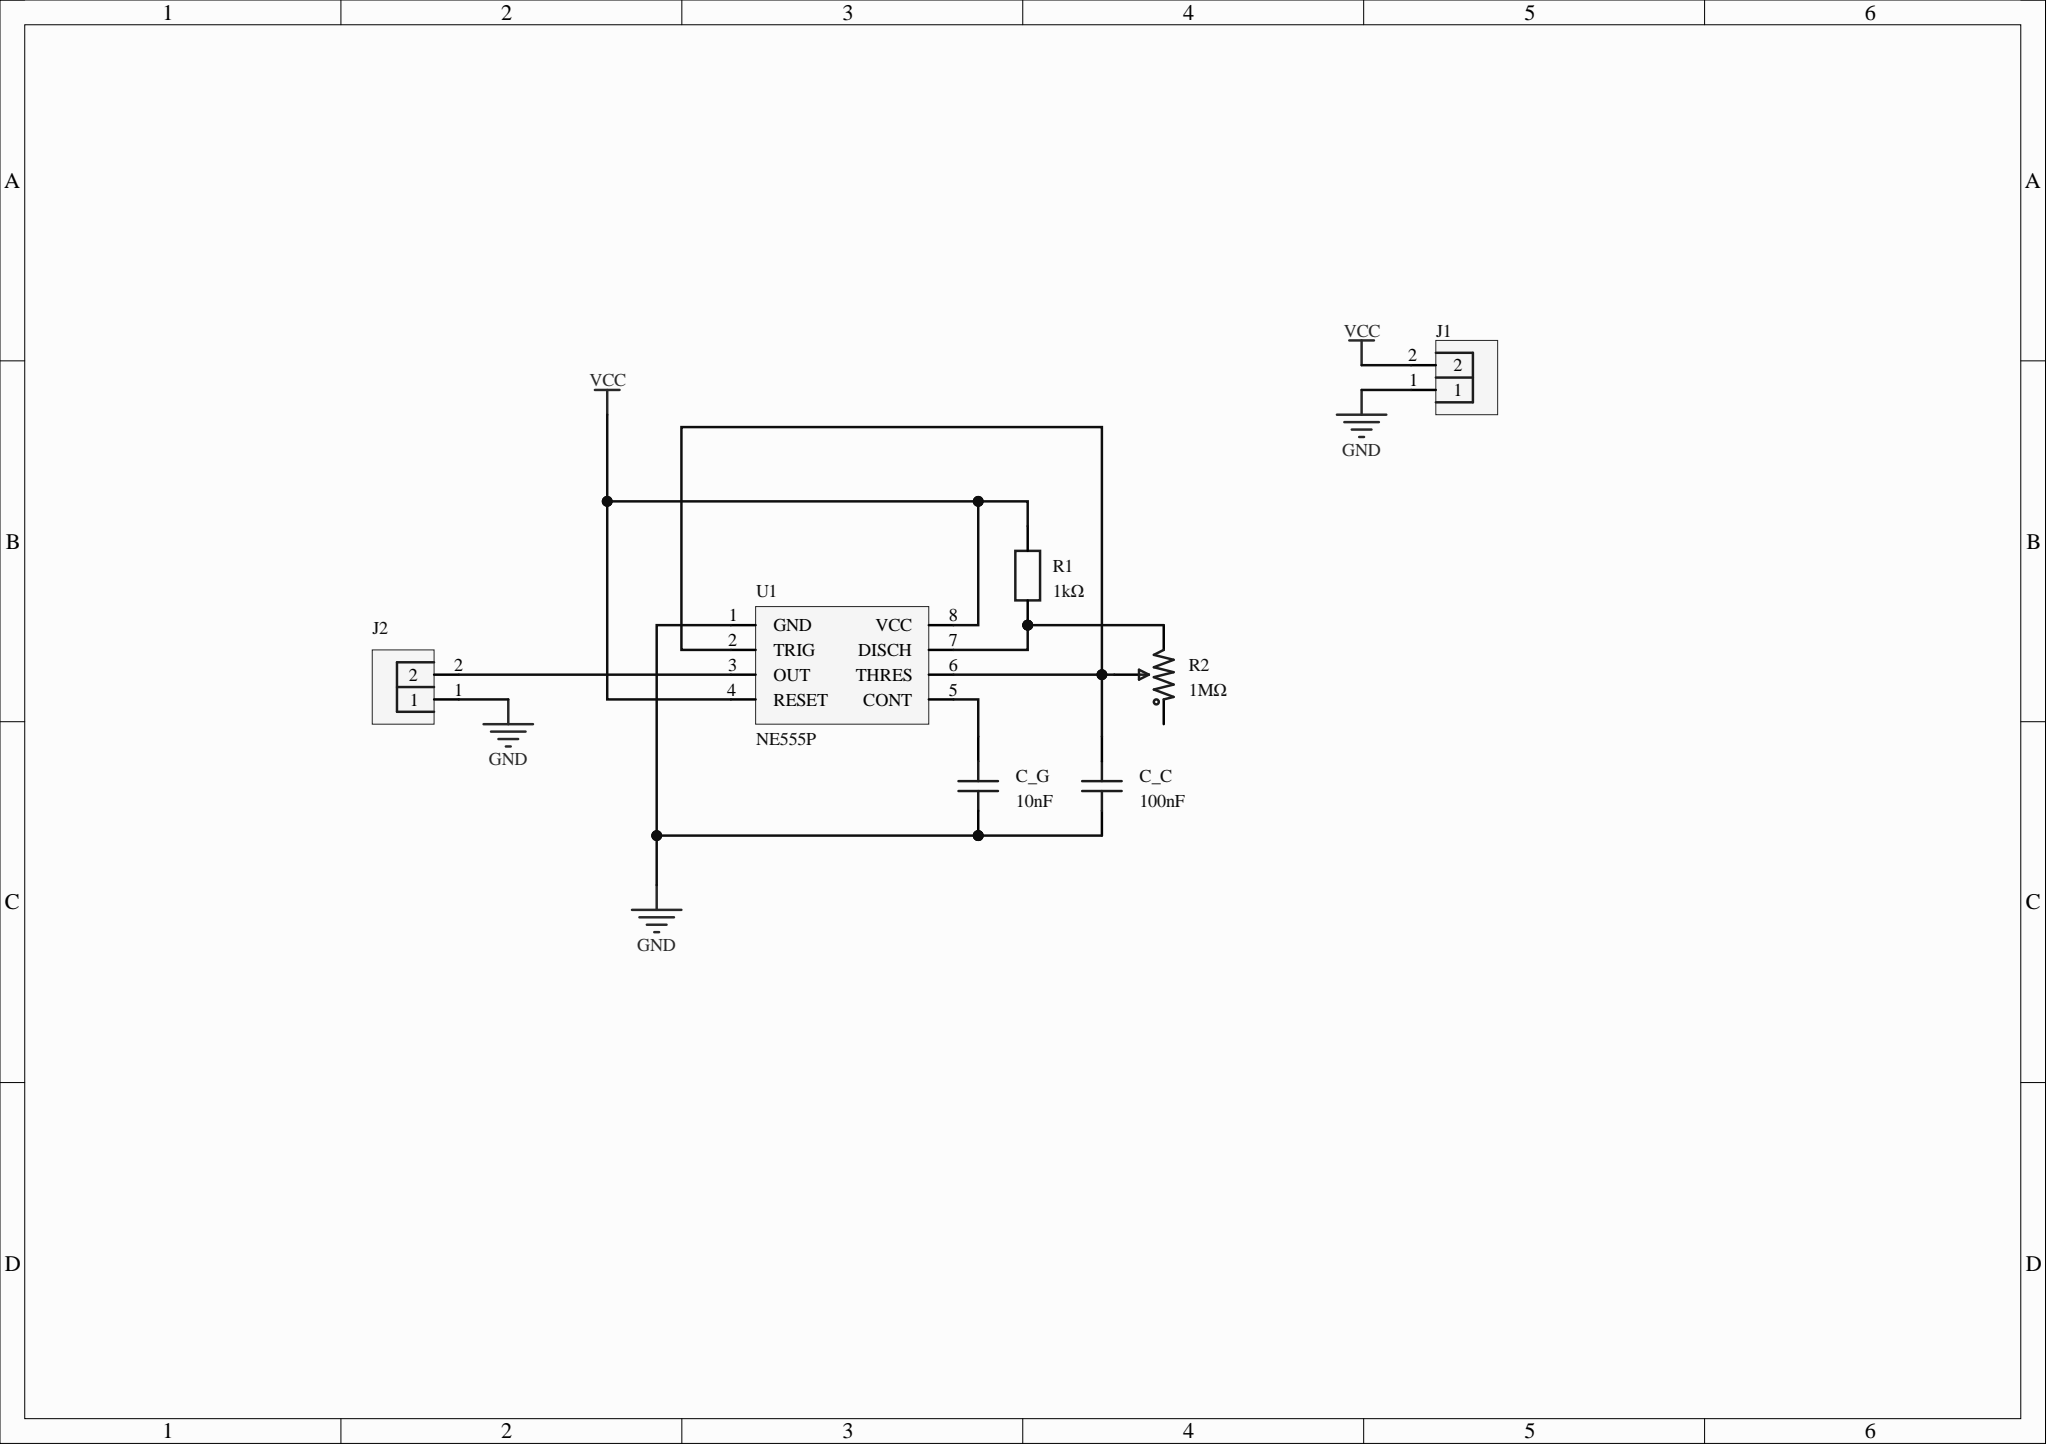Circuit board | Altium Designer | 7 parts | 6 nets
Bill of materials:
Comment,Description,Designator,Footprint,LibRef,Quantity
"100nF","Capacitance: 100nF; tolerance: ±20%; rated voltage: 50V; temperature coefficient: Y5V;","C_C","CAP-TH_L5.0-W2.5-P5.00-D1.0","CC1H104MC1FD3F6C10MF","1"
"10nF","Capacitance: 10nF; tolerance: ±20%; rated voltage: 50V; temperature coefficient: Y5U;","C_G","CAP-TH_L5.5-W3.0-P5.00-D0.6","DCT103M22Y5UF6FJ5A0","1"
"","","J1, J2","HDR-TH_2P-P2.54-V-M-1","HDR-M_2.54_1x2P","2"
"1kΩ","Resistor type: metal film resistor; resistance: 1kΩ; tolerance: ±1%; power: 250mW; temperature coefficient: ±100ppm/?;","R1","RES-TH_BD2.7-L6.2-P10.20-D0.4","MF1/4W-1K±1%-ST52","1"
"1MΩ","Resistance: 1MΩ; tolerance: ±25%; power: 100mW;","R2","RES-ADJ-TH_RM063-103","RM063-105(1M)","1"
"NE555P","Precision timing circuits that generate accurate time delays or oscillations. In delay or monostable mode, the timing interval is set by a single external resistor and capacitor network. In astable mode, frequency and duty cycle are set by two external resistors and one external capacitor.","U1","DIP-8_L9.8-W6.6-P2.54-LS7.6-BL","NE555P","1"
Netlist (Protel format):
[
C_C
CAP-TH_L5.0-W2.5-P5.00-D1.0
100nF



]
[
C_G
CAP-TH_L5.5-W3.0-P5.00-D0.6
10nF



]
[
J1
HDR-TH_2P-P2.54-V-M-1




]
[
J2
HDR-TH_2P-P2.54-V-M-1




]
[
R1
RES-TH_BD2.7-L6.2-P10.20-D0.4
1kΩ



]
[
R2
RES-ADJ-TH_RM063-103
1MΩ



]
[
U1
DIP-8_L9.8-W6.6-P2.54-LS7.6-BL
NE555P



]
(
VCC
J1-2
R1-2
U1-4
U1-8
)
(
NetR1_1
R1-1
R2-3
U1-7
)
(
NetJ2_2
J2-2
U1-3
)
(
NetC_G_2
C_G-2
U1-5
)
(
NetC_C_2
C_C-2
R2-2
U1-2
U1-6
)
(
GND
C_C-1
C_G-1
J1-1
J2-1
U1-1
)